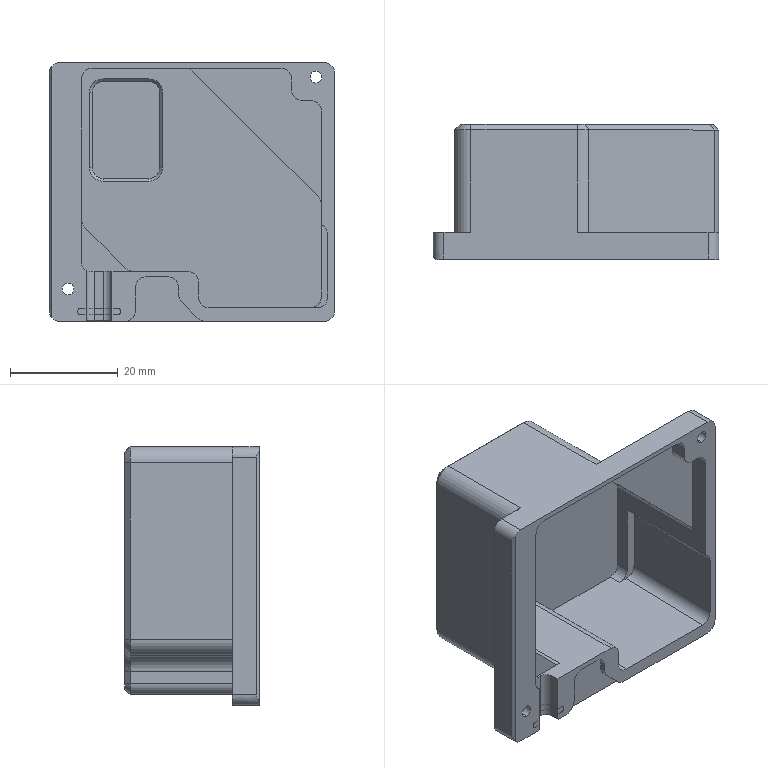NC program | NX | posted with a generic post | part box 53 x 25 x 48 mm
Whole program:
N10 G17 G21 G94 G90
(PLANAR_MILL , TOOL : D63面刀)
N12 T01 M6
N14 G53
N16 G17 G0 G90 X61. Y0.5 B0. C0. S3500 M3
N18 G43 Z30. H1
N20 Z10.5
N22 G94 G1 Z8.5 F1000.
N24 X24.5
N26 X-24.5
N28 X-61.
N30 Z10.5
N32 G0 Z30.
N34 X61.
N36 Z9.
N38 G1 Z7.
N40 X24.5
N42 X-24.5
N44 X-61.
N46 Z9.
N48 G0 Z30.
N50 X61.
N52 Z7.5
N54 G1 Z5.5
N56 X24.5
N58 X-24.5
N60 X-61.
N62 Z7.5
N64 G0 Z30.
N66 X61.
N68 Z6.
N70 G1 Z4.
N72 X24.5
N74 X-24.5
N76 X-61.
N78 Z6.
N80 G0 Z30.
N82 X61.
N84 Z4.5
N86 G1 Z2.5
N88 X24.5
N90 X-24.5
N92 X-61.
N94 Z4.5
N96 G0 Z30.
N98 X61.
N100 Z3.
N102 G1 Z1.
N104 X24.5
N106 X-24.5
N108 X-61.
N110 Z3.
N112 G0 Z30.
N114 X61.
N116 Z2.1
N118 G1 Z0.1
N120 X24.5
N122 X-24.5
N124 X-61.
N126 Z2.1
N128 G0 Z30.
N130 M5
(动态粗 , TOOL : D10-30-D10-75-3T-ROUGH)
N132 T02 M6
N134 G53
N136 G17 G0 G90 X-23.893 Y-37.072 B0. C0. S5500 M3
N138 G43 Z30. H2
N140 Z-25.5
N142 G94 G1 X-23.894 Y-37.047 Z-25.656 F3000.
N144 X-23.895 Y-37.022 Z-25.718
N146 X-23.897 Y-36.997 Z-25.763
N148 X-23.898 Y-36.972 Z-25.8
N150 X-23.899 Y-36.947 Z-25.831
N152 X-23.9 Y-36.922 Z-25.857
N154 X-23.901 Y-36.897 Z-25.88
N156 X-23.902 Y-36.872 Z-25.9
N158 X-23.904 Y-36.847 Z-25.918
N160 X-23.905 Y-36.822 Z-25.933
N162 X-23.906 Y-36.797 Z-25.947
N164 X-23.907 Y-36.772 Z-25.958
N166 X-23.908 Y-36.747 Z-25.968
N168 X-23.909 Y-36.722 Z-25.977
N170 X-23.911 Y-36.697 Z-25.984
N172 X-23.912 Y-36.672 Z-25.99
N174 X-23.913 Y-36.647 Z-25.994
N176 X-23.914 Y-36.622 Z-25.997
N178 X-23.915 Y-36.597 Z-25.999
N180 X-23.916 Y-36.572 Z-26.
N182 X-23.992 Y-34.947
N184 G3 X-24.586 Y-34.074 R1.011
N186 X-27.07 Y-33.379 R9.411
N188 G2 X-30.532 Y-30.901 R6.062
N190 X-32.369 Y-26.242 R11.725
N192 X-32.94 Y-19.299 R42.214
N194 X-32.999 Y-5.199 R831.551
N196 G1 X-32.998 Y26.216
N198 G2 X-31.246 Y29.838 R5.344
N200 X-26.941 Y32.098 R9.763
N202 X-21.001 Y32.863 R28.395
N204 X-8.778 Y32.999 R317.439
N206 G1 X26.101
N208 G2 X29.872 Y31.245 R5.296
N210 X32.089 Y27.044 R9.618
N212 X32.861 Y21.106 R27.873
N214 X32.996 Y10.757 R273.985
N216 G1 X32.999 Y4.607
N218 X32.996 Y-26.266
N220 G2 X31.18 Y-29.935 R5.367
N222 X26.957 Y-32.112 R9.75
N224 X21.165 Y-32.859 R28.288
N226 X8.942 Y-32.999 R307.355
N228 G1 X-20.967
N230 G2 X-24.759 Y-32.572 R16.587
N232 X-29.481 Y-28.855 R8.179
N234 X-31.096 Y-24.827 R14.44
N236 G1 X-31.266 Y-24.461
N238 X-31.591 Y-23.249
N240 G2 X-31.968 Y-14.206 R102.092
N242 G1 X-31.999 Y-1.606
N244 Y23.141
N246 G2 X-29.1 Y28.834 R7.324
N248 X-24.15 Y31.093 R12.446
N250 X-17.679 Y31.856 R35.091
N252 X-4.781 Y31.998 R344.183
N254 G1 X23.116 Y31.999
N256 G2 X28.866 Y29.085 R7.297
N258 X30.66 Y25.721 R11.839
N260 G1 X31.266 Y24.461
N262 X31.591 Y23.249
N264 G2 X31.973 Y13.305 R113.748
N266 G1 X31.999 Y1.305
N268 X31.997 Y-23.266
N270 G2 X29.023 Y-28.915 R7.322
N272 X23.978 Y-31.14 R12.708
N274 X17.428 Y-31.869 R36.981
N276 X4.829 Y-31.998 R367.336
N278 G1 X-18.396 Y-31.999
N280 G2 X-22.281 Y-31.74 R21.075
N282 X-27.439 Y-28.595 R8.954
N284 G3 X-28.101 Y-28.235 R2.521
N286 G1 X-29.129 Y-27.515
N288 X-30.016 Y-26.627
N290 X-30.736 Y-25.599
N292 X-31.266 Y-24.461
N294 X-31.591 Y-23.249
N296 X-31.7 Y-21.999
N298 Y22.001
N300 X-31.59 Y23.252
N302 X-31.265 Y24.464
N304 X-30.735 Y25.601
N306 X-30.015 Y26.629
N308 X-29.127 Y27.516
N310 X-28.099 Y28.236
N312 G2 X-20.3 Y30.49 R22.982
N314 X-11.767 Y30.949 R81.081
N316 X2.183 Y30.999 R865.522
N318 G1 X20.533 Y30.998
N320 G2 X26.301 Y28.995 R8.611
N322 G3 X26.964 Y28.765 R2.303
N324 G1 X28.101 Y28.235
N326 X29.129 Y27.515
N328 X30.016 Y26.627
N330 X30.704 Y25.644
N332 X30.016 Y26.627
N334 X29.129 Y27.515
N336 X28.101 Y28.235
N338 X26.964 Y28.765
N340 G2 X24.7 Y29.488 R31.583
N342 G3 X19.447 Y30.275 R21.41
N344 X8.649 Y30.397 R262.12
N346 G1 X-20.601 Y30.398
N348 G3 X-21.378 Y30.129 R2.675
N350 G2 X-24.081 Y29.207 R35.926
N352 G3 X-25.749 Y29.091 R21.304
N354 G1 X-26.961 Y28.766
N356 X-25.749 Y29.091
N358 G2 X-23.106 Y29.2 R17.442
N360 X-13.118 Y29.391 R181.346
N362 G1 X-5.468 Y29.398
N364 X20.381 Y29.391
N366 X21.377 Y29.2
N368 X24.501
N370 X25.752 Y29.09
N372 X26.331 Y28.935
N374 X25.752 Y29.09
N376 X24.501 Y29.2
N378 X-23.173
N380 G2 X-23.891 Y30.895 R1.
N382 X-23.423 Y31.173 Z-25.972 R1.136
N384 G1 X-22.092 Y31.652 Z-25.9
N386 X-20.386 Y32.267 F15000.
N388 X-20.219 Y32.309
N390 X-20.047 Y32.326
N392 X24.345
N394 G2 X28.71 Y31.457 R11.411
N396 G1 X29.351 Y31.193
N398 X29.987 Y30.918
N400 G2 X32.73 Y28.35 R6.433
N402 G1 X32.895 Y28.045
N404 X33.048 Y27.734
N406 X33.91 Y25.828
N408 G2 X33.749 Y24.754 R1.001
N410 G1 X32.468 Y23.264 Z-26. F3000.
N412 X32.156 Y22.906
N414 X31.857 Y22.537
N416 G3 X31.7 Y21.999 R1.012
N418 G1 Y-22.001
N420 X31.59 Y-23.252
N422 X31.265 Y-24.464
N424 X30.735 Y-25.601
N426 X30.015 Y-26.629
N428 X29.127 Y-27.516
N430 X28.099 Y-28.236
N432 G2 X20.303 Y-30.491 R22.898
N434 X11.919 Y-30.947 R79.781
N436 X-2.18 Y-30.999 R863.668
N438 G1 X-16.617 Y-30.997
N440 G2 X-20.65 Y-30.721 R20.837
N442 X-24.181 Y-29.297 R11.527
N444 G1 X-24.501 Y-29.2
N446 X-25.752 Y-29.09
N448 X-26.964 Y-28.765
N450 X-27.643 Y-28.448
N452 X-26.964 Y-28.765
N454 X-25.752 Y-29.09
N456 G2 X-23.975 Y-29.273 R15.572
N458 G3 X-16.479 Y-30.322 R29.375
N460 X-5.23 Y-30.398 R486.369
N462 G1 X20.426 Y-30.392
N464 G3 X21.594 Y-29.977 R14.303
N466 G1 X24.003 Y-29.209
N468 G3 X25.749 Y-29.091 R19.671
N470 G1 X26.961 Y-28.766
N472 X25.749 Y-29.091
N474 G2 X22.877 Y-29.2 R19.176
N476 X12.945 Y-29.391 R180.349
N478 G1 X5.295 Y-29.398
N480 X-19.401 Y-29.391
N482 X-20.246 Y-29.2
N484 X-24.446
N486 X22.879
N488 G2 X23.889 Y-30.195 R1.01
N490 G1 X23.912 Y-31.656
N492 Y-31.681 Z-25.999
N494 Y-31.706 Z-25.997
N496 X23.913 Y-31.731 Z-25.994
N498 Y-31.756 Z-25.99
N500 Y-31.781 Z-25.984
N502 X23.914 Y-31.806 Z-25.977
N504 Y-31.831 Z-25.968
N506 X23.915 Y-31.856 Z-25.958
N508 Y-31.881 Z-25.947
N510 Y-31.906 Z-25.933
N512 X23.916 Y-31.931 Z-25.918
N514 Y-31.956 Z-25.9
N516 X23.917 Y-31.981 Z-25.88
N518 Y-32.006 Z-25.857
N520 Y-32.031 Z-25.831
N522 X23.918 Y-32.056 Z-25.8
N524 Y-32.081 Z-25.763
N526 Y-32.106 Z-25.718
N528 X23.919 Y-32.131 Z-25.656
N530 Y-32.156 Z-25.5
N532 G0 Z30.
N534 X34.653 Y2.366
N536 Z-19.35
N538 G1 X34.628 Y2.368 Z-19.506
N540 X34.603 Y2.371 Z-19.568
N542 X34.579 Y2.373 Z-19.613
N544 X34.554 Y2.376 Z-19.65
N546 X34.529 Y2.378 Z-19.681
N548 X34.504 Y2.381 Z-19.707
N550 X34.479 Y2.383 Z-19.73
N552 X34.454 Y2.386 Z-19.75
N554 X34.429 Y2.388 Z-19.768
N556 X34.404 Y2.391 Z-19.783
N558 X34.38 Y2.393 Z-19.797
N560 X34.355 Y2.396 Z-19.808
N562 X34.33 Y2.399 Z-19.818
N564 X34.305 Y2.401 Z-19.827
N566 X34.28 Y2.404 Z-19.834
N568 X34.255 Y2.406 Z-19.84
N570 X34.23 Y2.409 Z-19.844
N572 X34.205 Y2.411 Z-19.847
N574 X34.181 Y2.414 Z-19.849
N576 X34.156 Y2.416 Z-19.85
N578 X32.761 Y2.559
N580 G3 X31.652 Y1.633 R1.01
N582 G1 X31.599 Y0.959
N584 G3 X30.838 Y-4.394 R22.716
N586 X30.702 Y-15.394 R279.85
N588 G2 X30.654 Y-20.416 R96.254
N590 X26.66 Y-26.424 R7.015
N592 X21.698 Y-27.799 R14.955
N594 X13.986 Y-28.172 R71.25
N596 G1 X4.237 Y-28.213
N598 G3 X3.237 Y-28.639 R5.185
N600 G2 X0.949 Y-29.165 R9.06
N602 G3 X4.225 Y-28.177 R8.667
N604 G2 X7.235 Y-27.735 R12.393
N606 X15.718 Y-27.538 R294.625
N608 G3 X22.142 Y-27.03 R43.461
N610 X26.005 Y-25.652 R10.515
N612 X29.114 Y-21.433 R7.891
N614 X29.949 Y-16.493 R19.177
N616 X30.145 Y-7.9 R215.758
N618 G2 X30.487 Y-2.091 R50.157
N620 X30.806 Y-1.481 R2.357
N622 G1 X31.298 Y-0.292
N624 X30.806 Y-1.481
N626 G3 X29.663 Y-4.405 R6.731
N628 X29.175 Y-10.132 R40.84
N630 G2 X28.863 Y-16.631 R105.01
N632 X27.87 Y-20.691 R12.543
N634 X23.778 Y-24.634 R8.63
N636 X18.307 Y-26.139 R17.473
N638 X11.36 Y-26.581 R74.022
N640 G3 X6.179 Y-26.932 R44.532
N642 X5.409 Y-27.38 R1.542
N644 G2 X4.109 Y-28.229 R11.382
N646 G3 X5.798 Y-27.044 R8.102
N648 G2 X7.821 Y-26.397 R5.674
N650 X12.984 Y-25.946 R50.703
N652 G3 X19.392 Y-25.263 R44.429
N654 X23.965 Y-23.457 R12.353
N656 X27.348 Y-18.798 R9.244
N658 X28.332 Y-13.579 R21.195
N660 G2 X28.768 Y-7.08 R726.147
N662 X29.431 Y-3.451 R15.916
N664 X30.133 Y-2.578 R6.668
N666 G1 X30.329 Y-2.258
N668 G2 X29.54 Y-3.273 R5.867
N670 G3 X28.455 Y-5.357 R5.012
N672 X27.667 Y-10.098 R26.27
N674 G2 X26.997 Y-15.442 R53.679
N676 X25.13 Y-19.903 R10.878
N678 X20.306 Y-23.371 R10.748
N680 X14.685 Y-24.646 R23.675
N682 G3 X9.234 Y-25.255 R242.757
N684 X7.198 Y-25.726 R10.043
N686 G1 X6.98 Y-25.874
N688 X5.791 Y-27.05
N690 X7.142 Y-25.717
N692 G2 X9.308 Y-24.881 R6.256
N694 X14.206 Y-24.106 R63.927
N696 G3 X19.659 Y-22.782 R23.632
N698 X25.624 Y-16.653 R10.213
N700 X26.805 Y-11.625 R23.652
N702 G2 X27.613 Y-6.623 R61.922
N704 X28.305 Y-4.574 R8.773
N706 X29.298 Y-3.556 R41.327
N708 G1 X27.921 Y-4.956
N710 G3 X26.706 Y-7.744 R8.367
N712 X25.655 Y-12.512 R121.297
N714 G2 X23.918 Y-17.124 R15.184
N716 X18.821 Y-21.433 R11.225
N718 X13.508 Y-23.014 R25.164
N720 G3 X9.197 Y-23.999 R42.911
N722 X8.555 Y-24.299 R1.824
N724 G1 X7.07 Y-25.784
N726 X8.716 Y-24.143
N728 G2 X10.97 Y-23.136 R7.531
N730 G3 X15.59 Y-21.875 R653.743
N732 X20.541 Y-19.434 R14.929
N734 X24.237 Y-14.21 R12.038
N736 X25.699 Y-9.249 R45.366
N738 G2 X26.819 Y-6.059 R15.536
N740 X28.068 Y-4.786 R111.949
N742 G1 X26.367 Y-6.507
N744 G3 X24.939 Y-9.323 R10.522
N746 G2 X23.294 Y-13.576 R53.886
N748 X17.114 Y-19.77 R12.782
N750 X12.487 Y-21.562 R37.332
N752 G3 X10.566 Y-22.308 R12.017
N754 G1 X8.622 Y-24.232
N756 G2 X10.79 Y-22.093 R54.525
N758 X13.516 Y-20.7 R14.545
N760 G3 X18.011 Y-18.399 R25.808
N762 X22.65 Y-12.938 R13.976
N764 X24.532 Y-8.747 R134.023
N766 G2 X25.022 Y-7.832 R6.552
N768 G1 X26.507 Y-6.347
N770 G3 X24.194 Y-8.692 R58.579
N772 X22.278 Y-11.689 R28.412
N774 G2 X15.536 Y-18.342 R17.219
N776 G1 X13.288 Y-19.578
N778 X10.631 Y-22.223
N780 G2 X13.859 Y-19.031 R101.293
N782 G1 X17.007 Y-16.648
N784 G3 X21.488 Y-11.589 R21.689
N786 G1 X21.967 Y-10.887
N788 X24.407 Y-8.447
N790 X13.535 Y-19.319
N792 G3 X13.443 Y-20.641 R1.01
N794 G1 X14.405 Y-21.917
N796 X14.42 Y-21.937 Z-19.849
N798 X14.435 Y-21.957 Z-19.847
N800 X14.45 Y-21.977 Z-19.844
N802 X14.465 Y-21.996 Z-19.84
N804 X14.48 Y-22.016 Z-19.834
N806 X14.495 Y-22.036 Z-19.827
N808 X14.51 Y-22.056 Z-19.818
N810 X14.525 Y-22.076 Z-19.808
N812 X14.54 Y-22.096 Z-19.797
N814 X14.556 Y-22.116 Z-19.783
N816 X14.571 Y-22.136 Z-19.768
N818 X14.586 Y-22.156 Z-19.75
N820 X14.601 Y-22.176 Z-19.73
N822 X14.616 Y-22.196 Z-19.707
N824 X14.631 Y-22.216 Z-19.681
N826 X14.646 Y-22.236 Z-19.65
N828 X14.661 Y-22.256 Z-19.613
N830 X14.676 Y-22.276 Z-19.568
N832 X14.691 Y-22.296 Z-19.506
N834 X14.706 Y-22.316 Z-19.35
N836 G0 Z30.
N838 X-19.439 Y-32.153
N840 Z-19.35
N842 G1 X-19.436 Y-32.128 Z-19.506
N844 X-19.433 Y-32.103 Z-19.568
N846 X-19.431 Y-32.078 Z-19.613
N848 X-19.428 Y-32.053 Z-19.65
N850 X-19.425 Y-32.028 Z-19.681
N852 X-19.422 Y-32.004 Z-19.707
N854 X-19.42 Y-31.979 Z-19.73
N856 X-19.417 Y-31.954 Z-19.75
N858 X-19.414 Y-31.929 Z-19.768
N860 X-19.412 Y-31.904 Z-19.783
N862 X-19.409 Y-31.879 Z-19.797
N864 X-19.406 Y-31.854 Z-19.808
N866 X-19.403 Y-31.83 Z-19.818
N868 X-19.401 Y-31.805 Z-19.827
N870 X-19.398 Y-31.78 Z-19.834
N872 X-19.395 Y-31.755 Z-19.84
N874 X-19.392 Y-31.73 Z-19.844
N876 X-19.39 Y-31.705 Z-19.847
N878 X-19.387 Y-31.681 Z-19.849
N880 X-19.384 Y-31.656 Z-19.85
N882 X-19.232 Y-30.272
N884 G3 X-20.166 Y-29.154 R1.01
N886 G2 X-22.072 Y-28.801 R9.007
N888 X-24.991 Y-28.053 R19.087
N890 X-29.083 Y-24.09 R7.361
N892 X-30.341 Y-19.093 R16.241
N894 X-30.672 Y-11.678 R76.363
N896 G1 X-30.7 Y-0.653
N898 X-30.698 Y19.347
N900 G2 X-29.835 Y23.414 R8.663
N902 X-26.368 Y26.553 R7.337
N904 X-21.377 Y27.833 R15.992
N906 X-14.038 Y28.167 R73.073
N908 G1 X-1.798 Y28.199
N910 X21.791 Y28.198
N912 G2 X25.798 Y27.394 R8.825
N914 G1 X26.751 Y26.831
N916 G2 X31.658 Y20.625 R7.16
N918 G3 X31.026 Y23.041 R7.301
N920 X26.628 Y26.878 R7.346
N922 X22.072 Y27.478 R21.707
N924 X11.424 Y27.598 R260.976
N926 G1 X-8.876 Y27.599
N928 G3 X-18.811 Y27.404 R185.141
N930 X-24.053 Y26.547 R21.648
N932 X-28.916 Y21.974 R7.534
N934 X-29.905 Y17.144 R16.317
N936 X-30.095 Y8.973 R119.606
N938 G1 X-30.099 Y-2.402
N940 G3 X-29.978 Y-15.226 R371.321
N942 X-29.283 Y-21.025 R29.064
N944 X-25.95 Y-26.073 R8.383
N946 G1 X-24.871 Y-27.197
N948 X-23.807 Y-27.978
N950 G3 X-21.739 Y-28.888 R9.515
N952 G2 X-25.848 Y-26.183 R8.468
N954 X-27.432 Y-23.096 R8.722
N956 X-28.833 Y-15.521 R29.511
N958 X-29.09 Y-4.652 R171.255
N960 X-29.038 Y13.398 R916.211
N962 X-28.55 Y18.618 R29.351
N964 X-24.245 Y24.382 R8.278
N966 X-18.827 Y26.061 R15.985
N968 X-15.847 Y26.39 R112.84
N970 X-14.517 Y26.912 R24.221
N972 X-12.499 Y27.2 R8.359
N974 G1 X24.501
N976 X25.577 Y27.119
N978 G3 X25.906 Y29.083 R1.
N980 G1 X25.64 Y29.153
N982 X23.74 Y29.652 Z-19.75
N984 X23.357 Y29.756 F15000.
N986 X22.97 Y29.846
N988 X22.842 Y29.854
N990 X-13.738 Y29.8
N992 G3 X-14.497 Y29.45 R1.002
N994 X-14.731 Y28.943 Z-19.779 R1.103 F3000.
N996 G1 X-15.058 Y27.583 Z-19.85
N998 X-15.13 Y27.271
N1000 X-15.217 Y26.964
N1002 G2 X-15.672 Y26.451 R1.005
N1004 X-17.556 Y25.833 R7.659
N1006 G3 X-21.884 Y24.598 R29.795
N1008 X-27.25 Y19.068 R9.069
N1010 X-28.275 Y13.86 R19.397
N1012 X-28.492 Y5.165 R121.788
N1014 G1 X-28.496 Y1.715
N1016 X-28.49 Y-16.976
N1018 G2 X-27.699 Y-19.996 R98.506
N1020 G3 X-27.619 Y-22.171 R15.601
N1022 G1 X-27.432 Y-23.096
N1024 G2 X-27.699 Y-21.116 R9.142
N1026 G1 X-27.7 Y11.751
N1028 G2 X-27.327 Y14.396 R13.7
N1030 X-25.969 Y18.67 R15.612
N1032 X-21.617 Y22.901 R10.285
N1034 X-18.321 Y24.349 R31.685
N1036 G3 X-17.896 Y24.767 R1.472
N1038 G2 X-15.831 Y26.365 R7.2
N1040 G3 X-18.171 Y24.409 R6.785
N1042 G2 X-20.166 Y23.091 R14.115
N1044 G3 X-23.876 Y20.035 R13.41
N1046 X-25.542 Y17.27 R13.321
N1048 G1 X-26.064 Y16.664
N1050 X-26.766 Y15.551
N1052 X-27.28 Y14.34
N1054 X-27.567 Y13.175
N1056 X-27.28 Y14.34
N1058 X-26.766 Y15.551
N1060 X-26.064 Y16.664
N1062 X-25.194 Y17.651
N1064 G3 X-23.073 Y19.534 R94.987
N1066 G2 X-19.492 Y22.227 R58.246
N1068 G3 X-19.066 Y22.954 R1.407
N1070 G2 X-18.097 Y24.502 R7.553
N1072 G3 X-19.258 Y22.432 R6.686
N1074 G2 X-20.75 Y20.83 R8.504
N1076 G1 X-22.301 Y19.451
N1078 G2 X-23.04 Y19.146 R18.43
N1080 G1 X-24.177 Y18.485
N1082 X-24.815 Y17.962
N1084 X-24.177 Y18.485
N1086 X-23.04 Y19.146
N1088 G3 X-20.898 Y20.086 R12.22
N1090 X-19.687 Y21.063 R4.446
N1092 X-19.435 Y21.936 R2.504
N1094 G1 X-19.205 Y22.571
N1096 G3 X-19.595 Y21.158 R6.158
N1098 G2 X-20.918 Y19.814 R3.034
N1100 G1 X-21.811 Y19.617
N1102 G3 X-20.48 Y19.919 R11.995
N1104 X-19.647 Y20.875 R1.24
N1106 G1 X-19.573 Y21.243
N1108 G2 X-19.82 Y20.384 R2.69
N1110 X-20.672 Y19.855 R1.239
N1112 X-21.838 Y20.528 R1.01
N1114 G1 X-22.329 Y22.018
N1116 X-22.337 Y22.042 Z-19.849
N1118 X-22.345 Y22.065 Z-19.847
N1120 X-22.353 Y22.089 Z-19.844
N1122 X-22.36 Y22.113 Z-19.84
N1124 X-22.368 Y22.137 Z-19.834
N1126 X-22.376 Y22.16 Z-19.827
N1128 X-22.384 Y22.184 Z-19.818
N1130 X-22.392 Y22.208 Z-19.808
N1132 X-22.4 Y22.232 Z-19.797
N1134 X-22.407 Y22.255 Z-19.783
N1136 X-22.415 Y22.279 Z-19.768
N1138 X-22.423 Y22.303 Z-19.75
N1140 X-22.431 Y22.327 Z-19.73
N1142 X-22.439 Y22.35 Z-19.707
N1144 X-22.446 Y22.374 Z-19.681
N1146 X-22.454 Y22.398 Z-19.65
N1148 X-22.462 Y22.422 Z-19.613
N1150 X-22.47 Y22.445 Z-19.568
N1152 X-22.478 Y22.469 Z-19.506
N1154 X-22.486 Y22.493 Z-19.35
N1156 G0 Z30.
N1158 M5
(动态粗_COPY , TOOL : D6-18-D6-50-3T-ROUGH)
N1160 T03 M6
N1162 G53
N1164 G17 G0 G90 X-21.388 Y19.692 B0. C0. S5500 M3
N1166 G43 Z30. H3
N1168 Z-12.5
N1170 G94 G1 X-21.381 Y19.668 Z-12.656 F2000.
N1172 X-21.373 Y19.644 Z-12.718
N1174 X-21.366 Y19.62 Z-12.763
N1176 X-21.359 Y19.596 Z-12.8
N1178 X-21.351 Y19.572 Z-12.831
N1180 X-21.344 Y19.548 Z-12.857
N1182 X-21.337 Y19.524 Z-12.88
N1184 X-21.33 Y19.5 Z-12.9
N1186 X-21.322 Y19.477 Z-12.918
N1188 X-21.315 Y19.453 Z-12.933
N1190 X-21.308 Y19.429 Z-12.947
N1192 X-21.3 Y19.405 Z-12.958
N1194 X-21.293 Y19.381 Z-12.968
N1196 X-21.286 Y19.357 Z-12.977
N1198 X-21.278 Y19.333 Z-12.984
N1200 X-21.271 Y19.309 Z-12.99
N1202 X-21.264 Y19.285 Z-12.994
N1204 X-21.257 Y19.261 Z-12.997
N1206 X-21.249 Y19.237 Z-12.999
N1208 X-21.242 Y19.213 Z-13.
N1210 X-20.962 Y18.295
N1212 G3 X-20.323 Y17.869 R0.606
N1214 X-17.712 Y19.678 R2.89
N1216 G1 X-17.641 Y20.598
N1218 X-17.725 Y19.541
N1220 G2 X-19.289 Y17.955 R2.45
N1222 G1 X-19.872 Y17.913
N1224 X-19.008 Y17.978
N1226 G3 X-17.714 Y19.099 R1.891
N1228 G1 X-17.7 Y19.724
N1230 G2 X-17.728 Y18.974 R3.315
N1232 X-18.854 Y17.95 R1.566
N1234 G1 X-19.192
N1236 G3 X-18.202 Y18.135 R1.602
N1238 X-17.7 Y19.158 R0.968
N1240 G2 X-17.793 Y18.461 R1.258
N1242 X-18.731 Y17.95 R0.951
N1244 G3 X-17.832 Y18.244 R1.008
N1246 X-17.7 Y18.783 R0.854
N1248 G2 X-18.331 Y17.957 R0.704
N1250 X-18.979 Y18.362 R0.606
N1252 G1 X-19.344 Y19.428
N1254 X-19.353 Y19.452 Z-12.999
N1256 X-19.361 Y19.475 Z-12.997
N1258 X-19.369 Y19.499 Z-12.994
N1260 X-19.377 Y19.523 Z-12.99
N1262 X-19.385 Y19.546 Z-12.984
N1264 X-19.393 Y19.57 Z-12.977
N1266 X-19.401 Y19.593 Z-12.968
N1268 X-19.409 Y19.617 Z-12.958
N1270 X-19.417 Y19.641 Z-12.947
N1272 X-19.425 Y19.664 Z-12.933
N1274 X-19.434 Y19.688 Z-12.918
N1276 X-19.442 Y19.712 Z-12.9
N1278 X-19.45 Y19.735 Z-12.88
N1280 X-19.458 Y19.759 Z-12.857
N1282 X-19.466 Y19.783 Z-12.831
N1284 X-19.474 Y19.806 Z-12.8
N1286 X-19.482 Y19.83 Z-12.763
N1288 X-19.49 Y19.854 Z-12.718
N1290 X-19.498 Y19.877 Z-12.656
N1292 X-19.507 Y19.901 Z-12.5
N1294 G0 Z30.
N1296 X-20.53 Y19.836
N1298 Z-19.35
N1300 G1 X-20.528 Y19.811 Z-19.506
N1302 X-20.526 Y19.786 Z-19.568
N1304 X-20.524 Y19.761 Z-19.613
N1306 X-20.523 Y19.736 Z-19.65
N1308 X-20.521 Y19.711 Z-19.681
N1310 X-20.519 Y19.686 Z-19.707
N1312 X-20.517 Y19.661 Z-19.73
N1314 X-20.515 Y19.636 Z-19.75
N1316 X-20.514 Y19.611 Z-19.768
N1318 X-20.512 Y19.587 Z-19.783
N1320 X-20.51 Y19.562 Z-19.797
N1322 X-20.508 Y19.537 Z-19.808
N1324 X-20.506 Y19.512 Z-19.818
N1326 X-20.505 Y19.487 Z-19.827
N1328 X-20.503 Y19.462 Z-19.834
N1330 X-20.501 Y19.437 Z-19.84
N1332 X-20.499 Y19.412 Z-19.844
N1334 X-20.497 Y19.387 Z-19.847
N1336 X-20.495 Y19.362 Z-19.849
N1338 X-20.494 Y19.337 Z-19.85
N1340 X-20.432 Y18.483
N1342 G3 X-19.768 Y17.924 R0.606
N1344 X-17.883 Y19.118 R2.553
N1346 X-17.7 Y19.543 R0.91
N1348 G1 X-17.693 Y20.075
N1350 G2 X-17.729 Y19.32 R3.876
N1352 X-19.145 Y17.954 R2.18
N1354 G1 X-19.574 Y17.943
N1356 G3 X-18.705 Y18.025 R2.697
N1358 X-17.72 Y18.935 R1.667
N1360 G1 X-17.7 Y19.504
N1362 G2 X-17.77 Y18.732 R1.78
N1364 X-18.743 Y17.95 R1.364
N1366 G1 X-19.043
N1368 G3 X-18.03 Y18.19 R1.412
N1370 X-17.7 Y18.998 R0.802
N1372 G2 X-18.346 Y17.96 R0.908
N1374 G1 X-18.608 Y17.95
N1376 G3 X-17.796 Y18.276 R0.816
N1378 X-17.7 Y18.67 R1.149
N1380 X-18.209 Y19.268 R0.606
N1382 G1 X-19.194 Y19.428
N1384 X-19.219 Y19.432 Z-19.849
N1386 X-19.244 Y19.436 Z-19.847
N1388 X-19.268 Y19.44 Z-19.844
N1390 X-19.293 Y19.444 Z-19.84
N1392 X-19.318 Y19.448 Z-19.834
N1394 X-19.342 Y19.452 Z-19.827
N1396 X-19.367 Y19.456 Z-19.818
N1398 X-19.392 Y19.46 Z-19.808
N1400 X-19.416 Y19.464 Z-19.797
N1402 X-19.441 Y19.468 Z-19.783
N1404 X-19.466 Y19.472 Z-19.768
N1406 X-19.491 Y19.476 Z-19.75
N1408 X-19.515 Y19.48 Z-19.73
N1410 X-19.54 Y19.484 Z-19.707
N1412 X-19.565 Y19.488 Z-19.681
N1414 X-19.589 Y19.492 Z-19.65
N1416 X-19.614 Y19.496 Z-19.613
N1418 X-19.639 Y19.5 Z-19.568
N1420 X-19.663 Y19.504 Z-19.506
N1422 X-19.688 Y19.508 Z-19.35
N1424 G0 Z30.
(FLOOR_FACING , TOOL : D6-18-D6-50-3T-ROUGH)
N1426 X-5.615 Y2.403 S4500
N1428 Z2.8
N1430 G3 X-5.615 Y2.403 Z1.911 I2.7 J0.012 F1000.
N1432 X-5.615 Y2.403 Z1.022 I2.7 J0.012
N1434 X-5.615 Y2.403 Z0.133 I2.7 J0.012
N1436 X-1.006 Y0.506 Z-0.2 R2.7
N1438 G1 X1.389 Y2.9
N1440 X4.438 Y4.163
N1442 X1.389 Y2.9
N1444 X-0.582
N1446 G2 X-3.4 Y0.209 R21.1
N1448 G1 Y-1.889
N1450 X-4.663 Y-4.938
N1452 X-3.4 Y-1.889
N1454 X-1.006 Y0.506
N1456 X2.176 Y-2.676
N1458 X11.9 Y7.048
N1460 Y7.4
N1462 X-2.784
N1464 G2 X-7.9 Y2.551 R16.6
N1466 G1 Y-9.4
N1468 X-4.548
N1470 X2.176 Y-2.676
N1472 X5.358 Y-5.858
N1474 X16.4 Y5.184
N1476 Y11.9
N1478 X-5.415
N1480 G2 X-12.4 Y5.366 R12.1
N1482 G1 Y-13.9
N1484 X-2.684
N1486 X5.358 Y-5.858
N1488 X8.54 Y-9.04
N1490 X20.9 Y3.32
N1492 Y16.4
N1494 X-8.908
N1496 G2 X-16.5 Y9.15 R7.6
N1498 G1 X-16.9
N1500 Y-18.4
N1502 X-0.82
N1504 X8.54 Y-9.04
N1506 X9.247 Y-8.333
N1508 Z2.8
N1510 G0 Z30.
(FLOOR_FACING_COPY , TOOL : D6-18-D6-50-3T-ROUGH)
N1512 X-5.615 Y2.403
N1514 Z2.7
N1516 G3 X-5.615 Y2.403 Z1.811 I2.7 J0.012 F800.
N1518 X-5.615 Y2.403 Z0.922 I2.7 J0.012
N1520 X-5.615 Y2.403 Z0.033 I2.7 J0.012
N1522 X-1.006 Y0.506 Z-0.3 R2.7
N1524 G1 X1.389 Y2.9
N1526 X4.438 Y4.163
N1528 X1.389 Y2.9
N1530 X-0.582
N1532 G2 X-3.4 Y0.209 R21.1
N1534 G1 Y-1.889
N1536 X-4.663 Y-4.938
N1538 X-3.4 Y-1.889
N1540 X-1.006 Y0.506
N1542 X2.176 Y-2.676
N1544 X11.9 Y7.048
N1546 Y7.4
N1548 X-2.784
N1550 G2 X-7.9 Y2.551 R16.6
N1552 G1 Y-9.4
N1554 X-4.548
N1556 X2.176 Y-2.676
N1558 X5.358 Y-5.858
N1560 X16.4 Y5.184
N1562 Y11.9
N1564 X-5.415
N1566 G2 X-12.4 Y5.366 R12.1
N1568 G1 Y-13.9
N1570 X-2.684
N1572 X5.358 Y-5.858
N1574 X8.54 Y-9.04
N1576 X20.9 Y3.32
N1578 Y16.4
N1580 X-8.908
N1582 G2 X-16.5 Y9.15 R7.6
N1584 G1 X-16.9
N1586 Y-18.4
N1588 X-0.82
N1590 X8.54 Y-9.04
N1592 X9.247 Y-8.333
N1594 Z2.7
N1596 G0 Z30.
(PLANAR_MILL_1_COPY_COPY , TOOL : D6-18-D6-50-3T-ROUGH)
N1598 X-24.195 Y18.529
N1600 Z-8.
N1602 G1 Z-10. F600.
N1604 G3 X-21.618 Y17.364 R2.
N1606 G2 X-19.5 Y17.75 R6.
N1608 G1 X-17.5
N1610 Y20.
N1612 G2 X-17.116 Y21.922 R5.
N1614 G3 X-18.194 Y24.537 R2.
N1616 G1 X-24.195 Y18.529
N1618 G3 X-21.618 Y17.364 R2.
N1620 G2 X-19.5 Y17.75 R6.
N1622 G1 X-17.5
N1624 Y20.
N1626 G2 X-17.116 Y21.922 R5.
N1628 G3 X-18.194 Y24.537 R2.
N1630 G1 Z-8.
N1632 G0 Z30.
N1634 X-24.195 Y18.529
N1636 Z-18.
N1638 G1 Z-20.
N1640 G3 X-21.618 Y17.364 R2.
N1642 G2 X-19.5 Y17.75 R6.
N1644 G1 X-17.5
N1646 Y20.
N1648 G2 X-17.116 Y21.922 R5.
N1650 G3 X-18.194 Y24.537 R2.
N1652 G1 X-24.195 Y18.529
N1654 G3 X-21.618 Y17.364 R2.
N1656 G2 X-19.5 Y17.75 R6.
N1658 G1 X-17.5
N1660 Y20.
N1662 G2 X-17.116 Y21.922 R5.
N1664 G3 X-18.194 Y24.537 R2.
N1666 G1 Z-18.
N1668 G0 Z30.
N1670 M5
(FLOOR_FACING_COPY_COPY , TOOL : D3-9-D4-50-3T-FINISH)
N1672 T04 M6
N1674 G53
N1676 G17 G0 G90 X8. Y16. B0. C0. S4500 M3
N1678 G43 Z30. H4
N1680 Z1.7
N1682 G94 G1 Z-0.3 F800.
N1684 G3 X6. Y18. R2.
N1686 G1 X-10.5
N1688 Y16.75
N1690 G2 X-16.5 Y10.75 R6.
N1692 G1 X-18.5
N1694 Y-20.
N1696 X-0.157
N1698 X22.5 Y2.657
N1700 Y18.
N1702 X6.
N1704 X5.
N1706 G3 X3. Y16. R2.
N1708 G1 Z1.7
N1710 G0 Z30.
N1712 M5
(PLANAR_MILL_4 , TOOL : D10-30-D10-75-3T-FINISH)
N1714 T05 M6
N1716 G53
N1718 G17 G0 G90 X-13.5 Y-2.625 B0. C0. S4500 M3
N1720 G43 Z30. H5
N1722 Z2.
N1724 G94 G1 Z0. F800.
N1726 X-16.5
N1728 G3 X-18.5 Y-4.625 R2.
N1730 G1 Y-20.
N1732 X-0.157
N1734 X22.5 Y2.657
N1736 Y18.
N1738 X-10.5
N1740 Y17.75
N1742 G2 X-17.5 Y10.75 R7.
N1744 G1 X-18.5
N1746 Y-4.625
N1748 G3 X-16.5 Y-6.625 R2.
N1750 G1 X-13.5
N1752 Z2.
N1754 G0 Z30.
(PLANAR_MILL_1 , TOOL : D10-30-D10-75-3T-FINISH)
N1756 X22.5 Y31. S5500
N1758 Z-24.
N1760 G1 Z-26. F600.
N1762 G3 X24.5 Y29. R2.
N1764 G2 X31.5 Y22. R7.
N1766 G1 Y-22.
N1768 G2 X24.5 Y-29. R7.
N1770 G1 X-24.5
N1772 G2 X-31.5 Y-22. R7.
N1774 G1 Y22.
N1776 G2 X-24.5 Y29. R7.
N1778 G1 X24.5
N1780 G3 X26.5 Y31. R2.
N1782 G1 X22.5
N1784 G3 X24.5 Y29. R2.
N1786 G2 X31.5 Y22. R7.
N1788 G1 Y-22.
N1790 G2 X24.5 Y-29. R7.
N1792 G1 X-24.5
N1794 G2 X-31.5 Y-22. R7.
N1796 G1 Y22.
N1798 G2 X-24.5 Y29. R7.
N1800 G1 X24.5
N1802 G3 X26.5 Y31. R2.
N1804 G1 Z-24.
N1806 G0 Z30.
(PLANAR_MILL_1_COPY , TOOL : D10-30-D10-75-3T-FINISH)
N1808 X-17.5 Y-31. S4500
N1810 Z-18.
N1812 G1 Z-20. F800.
N1814 G3 X-19.5 Y-29. R2.
N1816 G2 X-27.5 Y-21. R8.
N1818 G1 Y11.75
N1820 G2 X-19.5 Y19.75 R8.
N1822 G1 Y20.
N1824 G2 X-12.5 Y27. R7.
N1826 G1 X24.5
N1828 G2 X31.5 Y20. R7.
N1830 G3 X33.5 Y18. R2.
N1832 G1 Z-18.
N1834 G0 Z30.
N1836 X-17.5 Y-31.
N1838 Z-18.
N1840 G1 Z-20.
N1842 G3 X-19.5 Y-29. R2.
N1844 G2 X-27.5 Y-21. R8.
N1846 G1 Y11.75
N1848 G2 X-19.5 Y19.75 R8.
N1850 G1 Y20.
N1852 G2 X-12.5 Y27. R7.
N1854 G1 X24.5
N1856 G2 X31.5 Y20. R7.
N1858 G3 X33.5 Y18. R2.
N1860 G1 Z-18.
N1862 G0 Z30.
N1864 Y4.243
N1866 Z-18.
N1868 G1 Z-20.
N1870 G3 X31.5 Y2.243 R2.
N1872 G2 X29.157 Y-3.414 R8.
N1874 G1 X5.914 Y-26.657
N1876 G2 X0.257 Y-29. R8.
N1878 G3 X-1.743 Y-31. R2.
N1880 G1 Z-18.
N1882 G0 Z30.
N1884 X33.5 Y4.243
N1886 Z-18.
N1888 G1 Z-20.
N1890 G3 X31.5 Y2.243 R2.
N1892 G2 X29.157 Y-3.414 R8.
N1894 G1 X5.914 Y-26.657
N1896 G2 X0.257 Y-29. R8.
N1898 G3 X-1.743 Y-31. R2.
N1900 G1 Z-18.
N1902 G0 Z30.
(PLANAR_MILL_1_COPY_COPY_1 , TOOL : D10-30-D10-75-3T-FINISH)
N1904 X32.864 Y-13.414
N1906 Z-18.
N1908 G1 Z-20.
N1910 G3 X30.036 Y-13.414 R2.
N1912 G1 X15.914 Y-27.536
N1914 G3 X15.914 Y-30.364 R2.
N1916 G1 Z-18.
N1918 G0 Z30.
N1920 X-33.011 Y19.545
N1922 Z-18.
N1924 G1 Z-20.
N1926 G3 X-30.187 Y19.693 R2.
N1928 G1 X-23.247 Y27.401
N1930 G3 X-23.395 Y30.225 R2.
N1932 G1 Z-18.
N1934 G0 Z30.
N1936 M5
(PLANAR_MILL_2 , TOOL : 倒角D6-90度)
N1938 T06 M6
N1940 G53
N1942 G17 G0 G90 X-25. Y-23. B0. C0. S3500 M3
N1944 G43 Z30. H6
N1946 Z0.5
N1948 G94 G1 Z-1.5 F800.
N1950 G3 X-23. Y-21. R2.
N1952 G1 Y11.75
N1954 G2 X-19.5 Y15.25 R3.5
N1956 G1 X-17.5
N1958 G3 X-15. Y17.75 R2.5
N1960 G1 Y20.
N1962 G2 X-12.5 Y22.5 R2.5
N1964 G1 X24.5
N1966 G2 X27. Y20. R2.5
N1968 G1 Y2.243
N1970 G2 X25.975 Y-0.232 R3.5
N1972 G1 X2.732 Y-23.475
N1974 G2 X0.257 Y-24.5 R3.5
N1976 G1 X-19.5
N1978 G2 X-23. Y-21. R3.5
N1980 G3 X-25. Y-19. R2.
N1982 G1 Z0.5
N1984 G0 Z30.
(PLANAR_MILL_2_COPY , TOOL : 倒角D6-90度)
N1986 X-22.5 Y-28.
N1988 Z-20.
N1990 G1 Z-22.
N1992 G3 X-24.5 Y-26. R2.
N1994 G2 X-28.5 Y-22. R4.
N1996 G1 Y22.
N1998 G2 X-24.5 Y26. R4.
N2000 G1 X24.5
N2002 G3 X26.5 Y28. R2.
N2004 G1 Z-20.
N2006 G0 Z30.
N2008 X30.5 Y0.
N2010 Z-20.
N2012 G1 Z-22.
N2014 G3 X28.5 Y-2. R2.
N2016 G1 Y-22.
N2018 G2 X24.5 Y-26. R4.
N2020 G1 X4.5
N2022 G3 X2.5 Y-28. R2.
N2024 G1 Z-20.
N2026 G0 Z30.
(DRILLING , TOOL : 倒角D6-90度)
N2028 X-23. Y18. S3000
N2030 G81 G98 Z-22.2 F200. R-17.
N2032 X23. Y-21.3
N2034 G80
N2036 G0 X23. Y-21.3 Z30.
N2038 M5
(DRILLING_COPY , TOOL : D2.2钻头)
N2040 T07 M6
N2042 G53
N2044 G17 G0 G90 X-23. Y18. B0. C0. S3000 M3
N2046 G43 Z30. H7
N2048 G94 G81 G98 Z-27.5 F150. R-17.
N2050 X23. Y-21.3
N2052 G80
N2054 G0 X23. Y-21.3 Z30.
N2056 M5
(HOLE_MILLING , TOOL : D3-9-D4-50-3T-FINISH)
N2058 T04 M6
N2060 G53
N2062 G17 G0 G90 X-23. Y18. B0. C0. S4500 M3
N2064 G43 Z30. H4
N2066 Z-19.5
N2068 G94 G3 X-22.65 Y17.65 R0.35 F300.
N2070 X-22.3 Y18. R0.35
N2072 X-22.3 Y18. Z-19.7 I-0.7 J0.
N2074 X-22.3 Y18. Z-19.9 I-0.7 J0.
N2076 X-22.3 Y18. Z-20.1 I-0.7 J0.
N2078 X-22.3 Y18. Z-20.3 I-0.7 J0.
N2080 X-22.3 Y18. Z-20.5 I-0.7 J0.
N2082 X-22.3 Y18. Z-20.7 I-0.7 J0.
N2084 X-22.3 Y18. Z-20.9 I-0.7 J0.
N2086 X-22.3 Y18. Z-21.1 I-0.7 J0.
N2088 X-22.3 Y18. Z-21.3 I-0.7 J0.
N2090 X-22.3 Y18. Z-21.5 I-0.7 J0.
N2092 X-22.3 Y18. Z-21.7 I-0.7 J0.
N2094 X-22.3 Y18. Z-21.9 I-0.7 J0.
N2096 X-23.7 Y18. Z-22. I-0.7 J0.
N2098 X-23. Y17.3 R0.7
N2100 X-23.7 Y18. R-0.7
N2102 X-23.35 Y17.65 R0.35
N2104 X-23. Y18. R0.35
N2106 G0 Z30.
N2108 X23. Y-21.3
N2110 Z-19.5
N2112 G3 X23.35 Y-21.65 R0.35
N2114 X23.7 Y-21.3 R0.35
N2116 X23.7 Y-21.3 Z-19.7 I-0.7 J0.
N2118 X23.7 Y-21.3 Z-19.9 I-0.7 J0.
N2120 X23.7 Y-21.3 Z-20.1 I-0.7 J0.
N2122 X23.7 Y-21.3 Z-20.3 I-0.7 J0.
N2124 X23.7 Y-21.3 Z-20.5 I-0.7 J0.
N2126 X23.7 Y-21.3 Z-20.7 I-0.7 J0.
N2128 X23.7 Y-21.3 Z-20.9 I-0.7 J0.
N2130 X23.7 Y-21.3 Z-21.1 I-0.7 J0.
N2132 X23.7 Y-21.3 Z-21.3 I-0.7 J0.
N2134 X23.7 Y-21.3 Z-21.5 I-0.7 J0.
N2136 X23.7 Y-21.3 Z-21.7 I-0.7 J0.
N2138 X23.7 Y-21.3 Z-21.9 I-0.7 J0.
N2140 X22.3 Y-21.3 Z-22. I-0.7 J0.
N2142 X23. Y-22. R0.7
N2144 X22.3 Y-21.3 R-0.7
N2146 X22.65 Y-21.65 R0.35
N2148 X23. Y-21.3 R0.35
N2150 G0 Z30.
N2152 M5
(PLANAR_MILL_2_COPY_1 , TOOL : 球刀R0.5-2-D4-50)
N2154 T08 M6
N2156 G53
N2158 G17 G0 G90 X-16.5 Y9.85 B0. C0. S3500 M3
N2160 G43 Z30. H8
N2162 Z1.8
N2164 G94 G1 Z-0.2 F800.
N2166 G3 X-18.5 Y11.85 R2.
N2168 X-19.6 Y10.75 R1.1
N2170 G1 Y-20.
N2172 G3 X-18.5 Y-21.1 R1.1
N2174 G1 X-0.157
N2176 G3 X0.621 Y-20.778 R1.1
N2178 G1 X23.278 Y1.879
N2180 G3 X23.6 Y2.657 R1.1
N2182 G1 Y18.
N2184 G3 X22.5 Y19.1 R1.1
N2186 G1 X-10.5
N2188 G3 X-11.6 Y18. R1.1
N2190 G1 Y16.75
N2192 G2 X-16.5 Y11.85 R4.9
N2194 G1 X-18.5
N2196 G3 X-19.5 Y10.85 R1.
N2198 G1 X-17.6 Y9.85
N2200 Z1.8
N2202 G0 Z30.
N2204 M5
N2206 M2